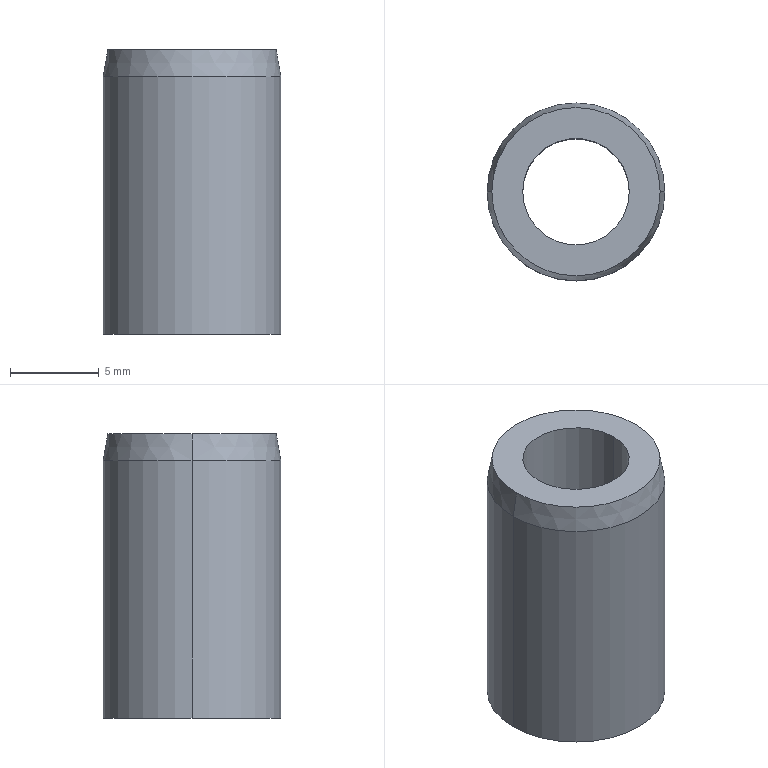Part | STEP file | Probe guide bush JBA6-16 | 1 solid | 10 faces | box 10 x 10 x 16 mm | volume 793.757 mm3 | cylinder 4 | spline 2 | cone 2 | plane 2 | commonest cylinder face diameters 6 x2 10 x2
STEP:
#1=CARTESIAN_POINT('',(0.,0.,0.));
#2=DIRECTION('',(0.,0.,1.));
#3=DIRECTION('',(1.,0.,0.));
#4=AXIS2_PLACEMENT_3D('',#1,#2,#3);
#5=CARTESIAN_POINT('',(4.,0.,0.));
#6=VERTEX_POINT('',#5);
#7=CARTESIAN_POINT('',(-4.,0.,0.));
#8=VERTEX_POINT('',#7);
#9=CARTESIAN_POINT('',(4.,0.,0.));
#10=CARTESIAN_POINT('',(4.,-8.,0.));
#11=CARTESIAN_POINT('',(-4.,-8.,0.));
#12=CARTESIAN_POINT('',(-4.,0.,0.));
#13=(BOUNDED_CURVE()B_SPLINE_CURVE(3,(#9,#10,#11,#12),.UNSPECIFIED.,.F.,.F.)B_SPLINE_CURVE_WITH_KNOTS((4,4),(0.,1.),.PIECEWISE_BEZIER_KNOTS.)CURVE()GEOMETRIC_REPRESENTATION_ITEM()RATIONAL_B_SPLINE_CURVE((1.,0.3333,0.3333,1.))REPRESENTATION_ITEM(''));
#14=CARTESIAN_POINT('',(-4.,0.,0.));
#15=CARTESIAN_POINT('',(-4.,-8.,0.));
#16=CARTESIAN_POINT('',(4.,-8.,0.));
#17=CARTESIAN_POINT('',(4.,0.,0.));
#18=CARTESIAN_POINT('',(-3.414,0.,0.));
#19=CARTESIAN_POINT('',(-3.414,-6.828,0.));
#20=CARTESIAN_POINT('',(3.414,-6.828,0.));
#21=CARTESIAN_POINT('',(3.414,0.,0.));
#22=CARTESIAN_POINT('',(-3.,0.,0.4142));
#23=CARTESIAN_POINT('',(-3.,-6.,0.4142));
#24=CARTESIAN_POINT('',(3.,-6.,0.4142));
#25=CARTESIAN_POINT('',(3.,0.,0.4142));
#26=CARTESIAN_POINT('',(-3.,0.,1.));
#27=CARTESIAN_POINT('',(-3.,-6.,1.));
#28=CARTESIAN_POINT('',(3.,-6.,1.));
#29=CARTESIAN_POINT('',(3.,0.,1.));
#30=(BOUNDED_SURFACE()B_SPLINE_SURFACE(3,3,((#14,#15,#16,#17),(#18,#19,#20,#21),(#22,#23,#24,#25),(#26,#27,#28,#29)),.UNSPECIFIED.,.F.,.F.,.F.)B_SPLINE_SURFACE_WITH_KNOTS((4,4),(4,4),(0.,1.),(0.,1.),.PIECEWISE_BEZIER_KNOTS.)GEOMETRIC_REPRESENTATION_ITEM()RATIONAL_B_SPLINE_SURFACE(((1.,0.3333,0.3333,1.),(0.8047,0.2682,0.2682,0.8047),(0.8047,0.2682,0.2682,0.8047),(1.,0.3333,0.3333,1.)))REPRESENTATION_ITEM('')SURFACE());
#31=CARTESIAN_POINT('',(0.,1.));
#32=DIRECTION('',(0.,-1.));
#33=VECTOR('',#32,1.);
#34=LINE('',#31,#33);
#35=(GEOMETRIC_REPRESENTATION_CONTEXT(2)PARAMETRIC_REPRESENTATION_CONTEXT()REPRESENTATION_CONTEXT('',''));
#36=DEFINITIONAL_REPRESENTATION('',(#34),#35);
#37=PCURVE('',#30,#36);
#38=CARTESIAN_POINT('',(0.,0.,0.));
#39=DIRECTION('',(0.,0.,1.));
#40=DIRECTION('',(1.,0.,0.));
#41=AXIS2_PLACEMENT_3D('',#38,#39,#40);
#42=PLANE('',#41);
#43=CARTESIAN_POINT('',(4.,0.));
#44=CARTESIAN_POINT('',(4.,-8.));
#45=CARTESIAN_POINT('',(-4.,-8.));
#46=CARTESIAN_POINT('',(-4.,0.));
#47=(BOUNDED_CURVE()B_SPLINE_CURVE(3,(#43,#44,#45,#46),.UNSPECIFIED.,.F.,.F.)B_SPLINE_CURVE_WITH_KNOTS((4,4),(0.,1.),.PIECEWISE_BEZIER_KNOTS.)CURVE()GEOMETRIC_REPRESENTATION_ITEM()RATIONAL_B_SPLINE_CURVE((1.,0.3333,0.3333,1.))REPRESENTATION_ITEM(''));
#48=(GEOMETRIC_REPRESENTATION_CONTEXT(2)PARAMETRIC_REPRESENTATION_CONTEXT()REPRESENTATION_CONTEXT('',''));
#49=DEFINITIONAL_REPRESENTATION('',(#47),#48);
#50=PCURVE('',#42,#49);
#51=SURFACE_CURVE('',#13,(#37,#50),.PCURVE_S1.);
#52=EDGE_CURVE('',#6,#8,#51,.T.);
#53=ORIENTED_EDGE('',*,*,#52,.T.);
#54=CARTESIAN_POINT('',(-3.,0.,1.));
#55=VERTEX_POINT('',#54);
#56=CARTESIAN_POINT('',(-4.,0.,1.));
#57=DIRECTION('',(0.,-1.,0.));
#58=DIRECTION('',(-1.,0.,0.));
#59=AXIS2_PLACEMENT_3D('',#56,#57,#58);
#60=CIRCLE('',#59,1.);
#61=CARTESIAN_POINT('',(0.,0.));
#62=CARTESIAN_POINT('',(0.01683,0.));
#63=CARTESIAN_POINT('',(0.04999,0.));
#64=CARTESIAN_POINT('',(0.09843,0.));
#65=CARTESIAN_POINT('',(0.1457,0.));
#66=CARTESIAN_POINT('',(0.192,0.));
#67=CARTESIAN_POINT('',(0.2375,0.));
#68=CARTESIAN_POINT('',(0.2823,0.));
#69=CARTESIAN_POINT('',(0.3265,0.));
#70=CARTESIAN_POINT('',(0.3703,0.));
#71=CARTESIAN_POINT('',(0.4137,0.));
#72=CARTESIAN_POINT('',(0.4569,0.));
#73=CARTESIAN_POINT('',(0.5,0.));
#74=CARTESIAN_POINT('',(0.5431,0.));
#75=CARTESIAN_POINT('',(0.5863,0.));
#76=CARTESIAN_POINT('',(0.6297,0.));
#77=CARTESIAN_POINT('',(0.6735,0.));
#78=CARTESIAN_POINT('',(0.7177,0.));
#79=CARTESIAN_POINT('',(0.7625,0.));
#80=CARTESIAN_POINT('',(0.808,0.));
#81=CARTESIAN_POINT('',(0.8543,0.));
#82=CARTESIAN_POINT('',(0.9016,0.));
#83=CARTESIAN_POINT('',(0.95,0.));
#84=CARTESIAN_POINT('',(0.9832,0.));
#85=CARTESIAN_POINT('',(1.,0.));
#86=B_SPLINE_CURVE_WITH_KNOTS('',3,(#61,#62,#63,#64,#65,#66,#67,#68,#69,#70,#71,#72,#73,#74,#75,#76,#77,#78,#79,#80,#81,#82,#83,#84,#85),.UNSPECIFIED.,.F.,.F.,(4,1,1,1,1,1,1,1,1,1,1,1,1,1,1,1,1,1,1,1,1,1,4),(1.571,1.642,1.714,1.785,1.856,1.928,1.999,2.071,2.142,2.213,2.285,2.356,2.428,2.499,2.57,2.642,2.713,2.785,2.856,2.927,2.999,3.07,3.142),.QUASI_UNIFORM_KNOTS.);
#87=(GEOMETRIC_REPRESENTATION_CONTEXT(2)PARAMETRIC_REPRESENTATION_CONTEXT()REPRESENTATION_CONTEXT('',''));
#88=DEFINITIONAL_REPRESENTATION('',(#86),#87);
#89=PCURVE('',#30,#88);
#90=CARTESIAN_POINT('',(4.,0.,0.));
#91=CARTESIAN_POINT('',(4.,8.,0.));
#92=CARTESIAN_POINT('',(-4.,8.,0.));
#93=CARTESIAN_POINT('',(-4.,0.,0.));
#94=CARTESIAN_POINT('',(3.414,0.,0.));
#95=CARTESIAN_POINT('',(3.414,6.828,0.));
#96=CARTESIAN_POINT('',(-3.414,6.828,0.));
#97=CARTESIAN_POINT('',(-3.414,0.,0.));
#98=CARTESIAN_POINT('',(3.,0.,0.4142));
#99=CARTESIAN_POINT('',(3.,6.,0.4142));
#100=CARTESIAN_POINT('',(-3.,6.,0.4142));
#101=CARTESIAN_POINT('',(-3.,0.,0.4142));
#102=CARTESIAN_POINT('',(3.,0.,1.));
#103=CARTESIAN_POINT('',(3.,6.,1.));
#104=CARTESIAN_POINT('',(-3.,6.,1.));
#105=CARTESIAN_POINT('',(-3.,0.,1.));
#106=(BOUNDED_SURFACE()B_SPLINE_SURFACE(3,3,((#90,#91,#92,#93),(#94,#95,#96,#97),(#98,#99,#100,#101),(#102,#103,#104,#105)),.UNSPECIFIED.,.F.,.F.,.F.)B_SPLINE_SURFACE_WITH_KNOTS((4,4),(4,4),(0.,1.),(0.,1.),.PIECEWISE_BEZIER_KNOTS.)GEOMETRIC_REPRESENTATION_ITEM()RATIONAL_B_SPLINE_SURFACE(((1.,0.3333,0.3333,1.),(0.8047,0.2682,0.2682,0.8047),(0.8047,0.2682,0.2682,0.8047),(1.,0.3333,0.3333,1.)))REPRESENTATION_ITEM('')SURFACE());
#107=CARTESIAN_POINT('',(0.,1.));
#108=CARTESIAN_POINT('',(0.01683,1.));
#109=CARTESIAN_POINT('',(0.04999,1.));
#110=CARTESIAN_POINT('',(0.09843,1.));
#111=CARTESIAN_POINT('',(0.1457,1.));
#112=CARTESIAN_POINT('',(0.192,1.));
#113=CARTESIAN_POINT('',(0.2375,1.));
#114=CARTESIAN_POINT('',(0.2823,1.));
#115=CARTESIAN_POINT('',(0.3265,1.));
#116=CARTESIAN_POINT('',(0.3703,1.));
#117=CARTESIAN_POINT('',(0.4137,1.));
#118=CARTESIAN_POINT('',(0.4569,1.));
#119=CARTESIAN_POINT('',(0.5,1.));
#120=CARTESIAN_POINT('',(0.5431,1.));
#121=CARTESIAN_POINT('',(0.5863,1.));
#122=CARTESIAN_POINT('',(0.6297,1.));
#123=CARTESIAN_POINT('',(0.6735,1.));
#124=CARTESIAN_POINT('',(0.7177,1.));
#125=CARTESIAN_POINT('',(0.7625,1.));
#126=CARTESIAN_POINT('',(0.808,1.));
#127=CARTESIAN_POINT('',(0.8543,1.));
#128=CARTESIAN_POINT('',(0.9016,1.));
#129=CARTESIAN_POINT('',(0.95,1.));
#130=CARTESIAN_POINT('',(0.9832,1.));
#131=CARTESIAN_POINT('',(1.,1.));
#132=B_SPLINE_CURVE_WITH_KNOTS('',3,(#107,#108,#109,#110,#111,#112,#113,#114,#115,#116,#117,#118,#119,#120,#121,#122,#123,#124,#125,#126,#127,#128,#129,#130,#131),.UNSPECIFIED.,.F.,.F.,(4,1,1,1,1,1,1,1,1,1,1,1,1,1,1,1,1,1,1,1,1,1,4),(1.571,1.642,1.714,1.785,1.856,1.928,1.999,2.071,2.142,2.213,2.285,2.356,2.428,2.499,2.57,2.642,2.713,2.785,2.856,2.927,2.999,3.07,3.142),.QUASI_UNIFORM_KNOTS.);
#133=(GEOMETRIC_REPRESENTATION_CONTEXT(2)PARAMETRIC_REPRESENTATION_CONTEXT()REPRESENTATION_CONTEXT('',''));
#134=DEFINITIONAL_REPRESENTATION('',(#132),#133);
#135=PCURVE('',#106,#134);
#136=SURFACE_CURVE('',#60,(#89,#135),.PCURVE_S1.);
#137=EDGE_CURVE('',#8,#55,#136,.T.);
#138=ORIENTED_EDGE('',*,*,#137,.T.);
#139=CARTESIAN_POINT('',(3.,0.,1.));
#140=VERTEX_POINT('',#139);
#141=CARTESIAN_POINT('',(0.,0.,1.));
#142=DIRECTION('',(0.,0.,1.));
#143=DIRECTION('',(1.,0.,0.));
#144=AXIS2_PLACEMENT_3D('',#141,#142,#143);
#145=CIRCLE('',#144,3.);
#146=CARTESIAN_POINT('',(1.,0.));
#147=CARTESIAN_POINT('',(1.,0.02375));
#148=CARTESIAN_POINT('',(1.,0.06805));
#149=CARTESIAN_POINT('',(1.,0.1267));
#150=CARTESIAN_POINT('',(1.,0.1794));
#151=CARTESIAN_POINT('',(1.,0.2276));
#152=CARTESIAN_POINT('',(1.,0.2721));
#153=CARTESIAN_POINT('',(1.,0.3139));
#154=CARTESIAN_POINT('',(1.,0.3535));
#155=CARTESIAN_POINT('',(1.,0.3914));
#156=CARTESIAN_POINT('',(1.,0.4282));
#157=CARTESIAN_POINT('',(1.,0.4643));
#158=CARTESIAN_POINT('',(1.,0.5));
#159=CARTESIAN_POINT('',(1.,0.5357));
#160=CARTESIAN_POINT('',(1.,0.5718));
#161=CARTESIAN_POINT('',(1.,0.6086));
#162=CARTESIAN_POINT('',(1.,0.6465));
#163=CARTESIAN_POINT('',(1.,0.6861));
#164=CARTESIAN_POINT('',(1.,0.7279));
#165=CARTESIAN_POINT('',(1.,0.7724));
#166=CARTESIAN_POINT('',(1.,0.8206));
#167=CARTESIAN_POINT('',(1.,0.8733));
#168=CARTESIAN_POINT('',(1.,0.9319));
#169=CARTESIAN_POINT('',(1.,0.9763));
#170=CARTESIAN_POINT('',(1.,1.));
#171=B_SPLINE_CURVE_WITH_KNOTS('',3,(#146,#147,#148,#149,#150,#151,#152,#153,#154,#155,#156,#157,#158,#159,#160,#161,#162,#163,#164,#165,#166,#167,#168,#169,#170),.UNSPECIFIED.,.F.,.F.,(4,1,1,1,1,1,1,1,1,1,1,1,1,1,1,1,1,1,1,1,1,1,4),(3.142,3.284,3.427,3.57,3.713,3.856,3.998,4.141,4.284,4.427,4.57,4.712,4.855,4.998,5.141,5.284,5.426,5.569,5.712,5.855,5.998,6.14,6.283),.QUASI_UNIFORM_KNOTS.);
#172=(GEOMETRIC_REPRESENTATION_CONTEXT(2)PARAMETRIC_REPRESENTATION_CONTEXT()REPRESENTATION_CONTEXT('',''));
#173=DEFINITIONAL_REPRESENTATION('',(#171),#172);
#174=PCURVE('',#30,#173);
#175=CARTESIAN_POINT('',(0.,0.,16.));
#176=DIRECTION('',(0.,0.,-1.));
#177=DIRECTION('',(-1.,0.,0.));
#178=AXIS2_PLACEMENT_3D('',#175,#176,#177);
#179=CYLINDRICAL_SURFACE('',#178,3.);
#180=CARTESIAN_POINT('',(9.425,15.));
#181=DIRECTION('',(-1.,0.));
#182=VECTOR('',#181,1.);
#183=LINE('',#180,#182);
#184=(GEOMETRIC_REPRESENTATION_CONTEXT(2)PARAMETRIC_REPRESENTATION_CONTEXT()REPRESENTATION_CONTEXT('',''));
#185=DEFINITIONAL_REPRESENTATION('',(#183),#184);
#186=PCURVE('',#179,#185);
#187=SURFACE_CURVE('',#145,(#174,#186),.PCURVE_S1.);
#188=EDGE_CURVE('',#55,#140,#187,.T.);
#189=ORIENTED_EDGE('',*,*,#188,.T.);
#190=CARTESIAN_POINT('',(4.,0.,1.));
#191=DIRECTION('',(0.,1.,0.));
#192=DIRECTION('',(1.,0.,0.));
#193=AXIS2_PLACEMENT_3D('',#190,#191,#192);
#194=CIRCLE('',#193,1.);
#195=CARTESIAN_POINT('',(0.,1.));
#196=CARTESIAN_POINT('',(0.01683,1.));
#197=CARTESIAN_POINT('',(0.04999,1.));
#198=CARTESIAN_POINT('',(0.09843,1.));
#199=CARTESIAN_POINT('',(0.1457,1.));
#200=CARTESIAN_POINT('',(0.192,1.));
#201=CARTESIAN_POINT('',(0.2375,1.));
#202=CARTESIAN_POINT('',(0.2823,1.));
#203=CARTESIAN_POINT('',(0.3265,1.));
#204=CARTESIAN_POINT('',(0.3703,1.));
#205=CARTESIAN_POINT('',(0.4137,1.));
#206=CARTESIAN_POINT('',(0.4569,1.));
#207=CARTESIAN_POINT('',(0.5,1.));
#208=CARTESIAN_POINT('',(0.5431,1.));
#209=CARTESIAN_POINT('',(0.5863,1.));
#210=CARTESIAN_POINT('',(0.6297,1.));
#211=CARTESIAN_POINT('',(0.6735,1.));
#212=CARTESIAN_POINT('',(0.7177,1.));
#213=CARTESIAN_POINT('',(0.7625,1.));
#214=CARTESIAN_POINT('',(0.808,1.));
#215=CARTESIAN_POINT('',(0.8543,1.));
#216=CARTESIAN_POINT('',(0.9016,1.));
#217=CARTESIAN_POINT('',(0.95,1.));
#218=CARTESIAN_POINT('',(0.9832,1.));
#219=CARTESIAN_POINT('',(1.,1.));
#220=B_SPLINE_CURVE_WITH_KNOTS('',3,(#195,#196,#197,#198,#199,#200,#201,#202,#203,#204,#205,#206,#207,#208,#209,#210,#211,#212,#213,#214,#215,#216,#217,#218,#219),.UNSPECIFIED.,.F.,.F.,(4,1,1,1,1,1,1,1,1,1,1,1,1,1,1,1,1,1,1,1,1,1,4),(1.571,1.642,1.714,1.785,1.856,1.928,1.999,2.071,2.142,2.213,2.285,2.356,2.428,2.499,2.57,2.642,2.713,2.785,2.856,2.927,2.999,3.07,3.142),.QUASI_UNIFORM_KNOTS.);
#221=(GEOMETRIC_REPRESENTATION_CONTEXT(2)PARAMETRIC_REPRESENTATION_CONTEXT()REPRESENTATION_CONTEXT('',''));
#222=DEFINITIONAL_REPRESENTATION('',(#220),#221);
#223=PCURVE('',#30,#222);
#224=CARTESIAN_POINT('',(0.,0.));
#225=CARTESIAN_POINT('',(0.01683,0.));
#226=CARTESIAN_POINT('',(0.04999,0.));
#227=CARTESIAN_POINT('',(0.09843,0.));
#228=CARTESIAN_POINT('',(0.1457,0.));
#229=CARTESIAN_POINT('',(0.192,0.));
#230=CARTESIAN_POINT('',(0.2375,0.));
#231=CARTESIAN_POINT('',(0.2823,0.));
#232=CARTESIAN_POINT('',(0.3265,0.));
#233=CARTESIAN_POINT('',(0.3703,0.));
#234=CARTESIAN_POINT('',(0.4137,0.));
#235=CARTESIAN_POINT('',(0.4569,0.));
#236=CARTESIAN_POINT('',(0.5,0.));
#237=CARTESIAN_POINT('',(0.5431,0.));
#238=CARTESIAN_POINT('',(0.5863,0.));
#239=CARTESIAN_POINT('',(0.6297,0.));
#240=CARTESIAN_POINT('',(0.6735,0.));
#241=CARTESIAN_POINT('',(0.7177,0.));
#242=CARTESIAN_POINT('',(0.7625,0.));
#243=CARTESIAN_POINT('',(0.808,0.));
#244=CARTESIAN_POINT('',(0.8543,0.));
#245=CARTESIAN_POINT('',(0.9016,0.));
#246=CARTESIAN_POINT('',(0.95,0.));
#247=CARTESIAN_POINT('',(0.9832,0.));
#248=CARTESIAN_POINT('',(1.,0.));
#249=B_SPLINE_CURVE_WITH_KNOTS('',3,(#224,#225,#226,#227,#228,#229,#230,#231,#232,#233,#234,#235,#236,#237,#238,#239,#240,#241,#242,#243,#244,#245,#246,#247,#248),.UNSPECIFIED.,.F.,.F.,(4,1,1,1,1,1,1,1,1,1,1,1,1,1,1,1,1,1,1,1,1,1,4),(1.571,1.642,1.714,1.785,1.856,1.928,1.999,2.071,2.142,2.213,2.285,2.356,2.428,2.499,2.57,2.642,2.713,2.785,2.856,2.927,2.999,3.07,3.142),.QUASI_UNIFORM_KNOTS.);
#250=(GEOMETRIC_REPRESENTATION_CONTEXT(2)PARAMETRIC_REPRESENTATION_CONTEXT()REPRESENTATION_CONTEXT('',''));
#251=DEFINITIONAL_REPRESENTATION('',(#249),#250);
#252=PCURVE('',#106,#251);
#253=SURFACE_CURVE('',#194,(#223,#252),.PCURVE_S1.);
#254=EDGE_CURVE('',#6,#140,#253,.T.);
#255=ORIENTED_EDGE('',*,*,#254,.F.);
#256=EDGE_LOOP('',(#53,#138,#189,#255));
#257=FACE_BOUND('',#256,.T.);
#258=ADVANCED_FACE('',(#257),#30,.T.);
#259=CARTESIAN_POINT('',(-5.,0.,14.5));
#260=VERTEX_POINT('',#259);
#261=CARTESIAN_POINT('',(5.,0.,14.5));
#262=VERTEX_POINT('',#261);
#263=CARTESIAN_POINT('',(0.,0.,14.5));
#264=DIRECTION('',(0.,0.,-1.));
#265=DIRECTION('',(-1.,0.,0.));
#266=AXIS2_PLACEMENT_3D('',#263,#264,#265);
#267=CIRCLE('',#266,5.);
#268=CARTESIAN_POINT('',(0.,0.,16.));
#269=DIRECTION('',(0.,0.,-1.));
#270=DIRECTION('',(-1.,0.,0.));
#271=AXIS2_PLACEMENT_3D('',#268,#269,#270);
#272=CYLINDRICAL_SURFACE('',#271,5.);
#273=CARTESIAN_POINT('',(0.,1.5));
#274=DIRECTION('',(1.,0.));
#275=VECTOR('',#274,1.);
#276=LINE('',#273,#275);
#277=(GEOMETRIC_REPRESENTATION_CONTEXT(2)PARAMETRIC_REPRESENTATION_CONTEXT()REPRESENTATION_CONTEXT('',''));
#278=DEFINITIONAL_REPRESENTATION('',(#276),#277);
#279=PCURVE('',#272,#278);
#280=CARTESIAN_POINT('',(0.,0.,14.5));
#281=DIRECTION('',(0.,0.,-1.));
#282=DIRECTION('',(-1.,0.,0.));
#283=AXIS2_PLACEMENT_3D('',#280,#281,#282);
#284=CONICAL_SURFACE('',#283,5.,0.1745);
#285=CARTESIAN_POINT('',(0.,0.));
#286=DIRECTION('',(1.,0.));
#287=VECTOR('',#286,1.);
#288=LINE('',#285,#287);
#289=(GEOMETRIC_REPRESENTATION_CONTEXT(2)PARAMETRIC_REPRESENTATION_CONTEXT()REPRESENTATION_CONTEXT('',''));
#290=DEFINITIONAL_REPRESENTATION('',(#288),#289);
#291=PCURVE('',#284,#290);
#292=SURFACE_CURVE('',#267,(#279,#291),.PCURVE_S1.);
#293=EDGE_CURVE('',#260,#262,#292,.T.);
#294=ORIENTED_EDGE('',*,*,#293,.T.);
#295=CARTESIAN_POINT('',(5.,0.,0.));
#296=VERTEX_POINT('',#295);
#297=CARTESIAN_POINT('',(5.,0.,16.));
#298=DIRECTION('',(0.,0.,-1.));
#299=VECTOR('',#298,1.);
#300=LINE('',#297,#299);
#301=CARTESIAN_POINT('',(3.142,0.));
#302=DIRECTION('',(0.,1.));
#303=VECTOR('',#302,1.);
#304=LINE('',#301,#303);
#305=(GEOMETRIC_REPRESENTATION_CONTEXT(2)PARAMETRIC_REPRESENTATION_CONTEXT()REPRESENTATION_CONTEXT('',''));
#306=DEFINITIONAL_REPRESENTATION('',(#304),#305);
#307=PCURVE('',#272,#306);
#308=CARTESIAN_POINT('',(0.,0.,16.));
#309=DIRECTION('',(0.,0.,-1.));
#310=DIRECTION('',(-1.,0.,0.));
#311=AXIS2_PLACEMENT_3D('',#308,#309,#310);
#312=CYLINDRICAL_SURFACE('',#311,5.);
#313=CARTESIAN_POINT('',(3.142,0.));
#314=DIRECTION('',(0.,1.));
#315=VECTOR('',#314,1.);
#316=LINE('',#313,#315);
#317=(GEOMETRIC_REPRESENTATION_CONTEXT(2)PARAMETRIC_REPRESENTATION_CONTEXT()REPRESENTATION_CONTEXT('',''));
#318=DEFINITIONAL_REPRESENTATION('',(#316),#317);
#319=PCURVE('',#312,#318);
#320=SURFACE_CURVE('',#300,(#307,#319),.PCURVE_S1.);
#321=EDGE_CURVE('',#262,#296,#320,.T.);
#322=ORIENTED_EDGE('',*,*,#321,.T.);
#323=CARTESIAN_POINT('',(-5.,0.,0.));
#324=VERTEX_POINT('',#323);
#325=CARTESIAN_POINT('',(0.,0.,0.));
#326=DIRECTION('',(0.,0.,1.));
#327=DIRECTION('',(-1.,0.,0.));
#328=AXIS2_PLACEMENT_3D('',#325,#326,#327);
#329=CIRCLE('',#328,5.);
#330=CARTESIAN_POINT('',(6.283,16.));
#331=DIRECTION('',(-1.,0.));
#332=VECTOR('',#331,1.);
#333=LINE('',#330,#332);
#334=(GEOMETRIC_REPRESENTATION_CONTEXT(2)PARAMETRIC_REPRESENTATION_CONTEXT()REPRESENTATION_CONTEXT('',''));
#335=DEFINITIONAL_REPRESENTATION('',(#333),#334);
#336=PCURVE('',#272,#335);
#337=CARTESIAN_POINT('',(0.,0.));
#338=DIRECTION('',(-1.,0.));
#339=AXIS2_PLACEMENT_2D('',#337,#338);
#340=CIRCLE('',#339,5.);
#341=(GEOMETRIC_REPRESENTATION_CONTEXT(2)PARAMETRIC_REPRESENTATION_CONTEXT()REPRESENTATION_CONTEXT('',''));
#342=DEFINITIONAL_REPRESENTATION('',(#340),#341);
#343=PCURVE('',#42,#342);
#344=SURFACE_CURVE('',#329,(#336,#343),.PCURVE_S1.);
#345=EDGE_CURVE('',#296,#324,#344,.T.);
#346=ORIENTED_EDGE('',*,*,#345,.T.);
#347=CARTESIAN_POINT('',(-5.,0.,16.));
#348=DIRECTION('',(0.,0.,-1.));
#349=VECTOR('',#348,1.);
#350=LINE('',#347,#349);
#351=CARTESIAN_POINT('',(0.,0.));
#352=DIRECTION('',(0.,1.));
#353=VECTOR('',#352,1.);
#354=LINE('',#351,#353);
#355=(GEOMETRIC_REPRESENTATION_CONTEXT(2)PARAMETRIC_REPRESENTATION_CONTEXT()REPRESENTATION_CONTEXT('',''));
#356=DEFINITIONAL_REPRESENTATION('',(#354),#355);
#357=PCURVE('',#272,#356);
#358=CARTESIAN_POINT('',(6.283,0.));
#359=DIRECTION('',(0.,1.));
#360=VECTOR('',#359,1.);
#361=LINE('',#358,#360);
#362=(GEOMETRIC_REPRESENTATION_CONTEXT(2)PARAMETRIC_REPRESENTATION_CONTEXT()REPRESENTATION_CONTEXT('',''));
#363=DEFINITIONAL_REPRESENTATION('',(#361),#362);
#364=PCURVE('',#312,#363);
#365=SURFACE_CURVE('',#350,(#357,#364),.PCURVE_S1.);
#366=EDGE_CURVE('',#260,#324,#365,.T.);
#367=ORIENTED_EDGE('',*,*,#366,.F.);
#368=EDGE_LOOP('',(#294,#322,#346,#367));
#369=FACE_BOUND('',#368,.T.);
#370=ADVANCED_FACE('',(#369),#272,.T.);
#371=CARTESIAN_POINT('',(-4.736,0.,16.));
#372=VERTEX_POINT('',#371);
#373=CARTESIAN_POINT('',(4.736,0.,16.));
#374=VERTEX_POINT('',#373);
#375=CARTESIAN_POINT('',(0.,0.,16.));
#376=DIRECTION('',(0.,0.,-1.));
#377=DIRECTION('',(-1.,0.,0.));
#378=AXIS2_PLACEMENT_3D('',#375,#376,#377);
#379=CIRCLE('',#378,4.736);
#380=CARTESIAN_POINT('',(0.,-1.5));
#381=DIRECTION('',(1.,0.));
#382=VECTOR('',#381,1.);
#383=LINE('',#380,#382);
#384=(GEOMETRIC_REPRESENTATION_CONTEXT(2)PARAMETRIC_REPRESENTATION_CONTEXT()REPRESENTATION_CONTEXT('',''));
#385=DEFINITIONAL_REPRESENTATION('',(#383),#384);
#386=PCURVE('',#284,#385);
#387=CARTESIAN_POINT('',(0.,0.,16.));
#388=DIRECTION('',(0.,0.,1.));
#389=DIRECTION('',(1.,0.,0.));
#390=AXIS2_PLACEMENT_3D('',#387,#388,#389);
#391=PLANE('',#390);
#392=CARTESIAN_POINT('',(-4.736,0.));
#393=CARTESIAN_POINT('',(-4.736,8.202));
#394=CARTESIAN_POINT('',(2.368,4.101));
#395=CARTESIAN_POINT('',(9.471,0.));
#396=CARTESIAN_POINT('',(2.368,-4.101));
#397=CARTESIAN_POINT('',(-4.736,-8.202));
#398=CARTESIAN_POINT('',(-4.736,0.));
#399=(BOUNDED_CURVE()B_SPLINE_CURVE(2,(#392,#393,#394,#395,#396,#397,#398),.UNSPECIFIED.,.T.,.F.)B_SPLINE_CURVE_WITH_KNOTS((1,2,2,2,2,1),(-2.094,0.,2.094,4.189,6.283,8.378),.UNSPECIFIED.)CURVE()GEOMETRIC_REPRESENTATION_ITEM()RATIONAL_B_SPLINE_CURVE((1.,0.5,1.,0.5,1.,0.5,1.))REPRESENTATION_ITEM(''));
#400=(GEOMETRIC_REPRESENTATION_CONTEXT(2)PARAMETRIC_REPRESENTATION_CONTEXT()REPRESENTATION_CONTEXT('',''));
#401=DEFINITIONAL_REPRESENTATION('',(#399),#400);
#402=PCURVE('',#391,#401);
#403=SURFACE_CURVE('',#379,(#386,#402),.PCURVE_S1.);
#404=EDGE_CURVE('',#372,#374,#403,.T.);
#405=ORIENTED_EDGE('',*,*,#404,.T.);
#406=CARTESIAN_POINT('',(5.,0.,14.5));
#407=DIRECTION('',(0.1736,0.,-0.9848));
#408=VECTOR('',#407,1.);
#409=LINE('',#406,#408);
#410=CARTESIAN_POINT('',(3.142,0.));
#411=DIRECTION('',(0.,1.));
#412=VECTOR('',#411,1.);
#413=LINE('',#410,#412);
#414=(GEOMETRIC_REPRESENTATION_CONTEXT(2)PARAMETRIC_REPRESENTATION_CONTEXT()REPRESENTATION_CONTEXT('',''));
#415=DEFINITIONAL_REPRESENTATION('',(#413),#414);
#416=PCURVE('',#284,#415);
#417=CARTESIAN_POINT('',(0.,0.,14.5));
#418=DIRECTION('',(0.,0.,-1.));
#419=DIRECTION('',(-1.,0.,0.));
#420=AXIS2_PLACEMENT_3D('',#417,#418,#419);
#421=CONICAL_SURFACE('',#420,5.,0.1745);
#422=CARTESIAN_POINT('',(3.142,0.));
#423=DIRECTION('',(0.,1.));
#424=VECTOR('',#423,1.);
#425=LINE('',#422,#424);
#426=(GEOMETRIC_REPRESENTATION_CONTEXT(2)PARAMETRIC_REPRESENTATION_CONTEXT()REPRESENTATION_CONTEXT('',''));
#427=DEFINITIONAL_REPRESENTATION('',(#425),#426);
#428=PCURVE('',#421,#427);
#429=SURFACE_CURVE('',#409,(#416,#428),.PCURVE_S1.);
#430=EDGE_CURVE('',#374,#262,#429,.T.);
#431=ORIENTED_EDGE('',*,*,#430,.T.);
#432=ORIENTED_EDGE('',*,*,#293,.F.);
#433=CARTESIAN_POINT('',(-5.,0.,14.5));
#434=DIRECTION('',(-0.1736,0.,-0.9848));
#435=VECTOR('',#434,1.);
#436=LINE('',#433,#435);
#437=CARTESIAN_POINT('',(0.,0.));
#438=DIRECTION('',(0.,1.));
#439=VECTOR('',#438,1.);
#440=LINE('',#437,#439);
#441=(GEOMETRIC_REPRESENTATION_CONTEXT(2)PARAMETRIC_REPRESENTATION_CONTEXT()REPRESENTATION_CONTEXT('',''));
#442=DEFINITIONAL_REPRESENTATION('',(#440),#441);
#443=PCURVE('',#284,#442);
#444=CARTESIAN_POINT('',(6.283,0.));
#445=DIRECTION('',(0.,1.));
#446=VECTOR('',#445,1.);
#447=LINE('',#444,#446);
#448=(GEOMETRIC_REPRESENTATION_CONTEXT(2)PARAMETRIC_REPRESENTATION_CONTEXT()REPRESENTATION_CONTEXT('',''));
#449=DEFINITIONAL_REPRESENTATION('',(#447),#448);
#450=PCURVE('',#421,#449);
#451=SURFACE_CURVE('',#436,(#443,#450),.PCURVE_S1.);
#452=EDGE_CURVE('',#372,#260,#451,.T.);
#453=ORIENTED_EDGE('',*,*,#452,.F.);
#454=EDGE_LOOP('',(#405,#431,#432,#453));
#455=FACE_BOUND('',#454,.T.);
#456=ADVANCED_FACE('',(#455),#284,.T.);
#457=CARTESIAN_POINT('',(-3.,0.,16.));
#458=VERTEX_POINT('',#457);
#459=CARTESIAN_POINT('',(-3.,0.,16.));
#460=DIRECTION('',(0.,0.,-1.));
#461=VECTOR('',#460,1.);
#462=LINE('',#459,#461);
#463=CARTESIAN_POINT('',(6.283,0.));
#464=DIRECTION('',(0.,1.));
#465=VECTOR('',#464,1.);
#466=LINE('',#463,#465);
#467=(GEOMETRIC_REPRESENTATION_CONTEXT(2)PARAMETRIC_REPRESENTATION_CONTEXT()REPRESENTATION_CONTEXT('',''));
#468=DEFINITIONAL_REPRESENTATION('',(#466),#467);
#469=PCURVE('',#179,#468);
#470=CARTESIAN_POINT('',(0.,0.,16.));
#471=DIRECTION('',(0.,0.,-1.));
#472=DIRECTION('',(-1.,0.,0.));
#473=AXIS2_PLACEMENT_3D('',#470,#471,#472);
#474=CYLINDRICAL_SURFACE('',#473,3.);
#475=CARTESIAN_POINT('',(0.,0.));
#476=DIRECTION('',(0.,1.));
#477=VECTOR('',#476,1.);
#478=LINE('',#475,#477);
#479=(GEOMETRIC_REPRESENTATION_CONTEXT(2)PARAMETRIC_REPRESENTATION_CONTEXT()REPRESENTATION_CONTEXT('',''));
#480=DEFINITIONAL_REPRESENTATION('',(#478),#479);
#481=PCURVE('',#474,#480);
#482=SURFACE_CURVE('',#462,(#469,#481),.PCURVE_S1.);
#483=EDGE_CURVE('',#458,#55,#482,.T.);
#484=ORIENTED_EDGE('',*,*,#483,.T.);
#485=ORIENTED_EDGE('',*,*,#188,.T.);
#486=CARTESIAN_POINT('',(3.,0.,16.));
#487=VERTEX_POINT('',#486);
#488=CARTESIAN_POINT('',(3.,0.,16.));
#489=DIRECTION('',(0.,0.,-1.));
#490=VECTOR('',#489,1.);
#491=LINE('',#488,#490);
#492=CARTESIAN_POINT('',(3.142,0.));
#493=DIRECTION('',(0.,1.));
#494=VECTOR('',#493,1.);
#495=LINE('',#492,#494);
#496=(GEOMETRIC_REPRESENTATION_CONTEXT(2)PARAMETRIC_REPRESENTATION_CONTEXT()REPRESENTATION_CONTEXT('',''));
#497=DEFINITIONAL_REPRESENTATION('',(#495),#496);
#498=PCURVE('',#179,#497);
#499=CARTESIAN_POINT('',(3.142,0.));
#500=DIRECTION('',(0.,1.));
#501=VECTOR('',#500,1.);
#502=LINE('',#499,#501);
#503=(GEOMETRIC_REPRESENTATION_CONTEXT(2)PARAMETRIC_REPRESENTATION_CONTEXT()REPRESENTATION_CONTEXT('',''));
#504=DEFINITIONAL_REPRESENTATION('',(#502),#503);
#505=PCURVE('',#474,#504);
#506=SURFACE_CURVE('',#491,(#498,#505),.PCURVE_S1.);
#507=EDGE_CURVE('',#487,#140,#506,.T.);
#508=ORIENTED_EDGE('',*,*,#507,.F.);
#509=CARTESIAN_POINT('',(0.,0.,16.));
#510=DIRECTION('',(0.,0.,-1.));
#511=DIRECTION('',(-1.,0.,0.));
#512=AXIS2_PLACEMENT_3D('',#509,#510,#511);
#513=CIRCLE('',#512,3.);
#514=CARTESIAN_POINT('',(0.,0.));
#515=DIRECTION('',(1.,0.));
#516=VECTOR('',#515,1.);
#517=LINE('',#514,#516);
#518=(GEOMETRIC_REPRESENTATION_CONTEXT(2)PARAMETRIC_REPRESENTATION_CONTEXT()REPRESENTATION_CONTEXT('',''));
#519=DEFINITIONAL_REPRESENTATION('',(#517),#518);
#520=PCURVE('',#179,#519);
#521=CARTESIAN_POINT('',(-3.,0.));
#522=CARTESIAN_POINT('',(-3.,5.196));
#523=CARTESIAN_POINT('',(1.5,2.598));
#524=CARTESIAN_POINT('',(6.,0.));
#525=CARTESIAN_POINT('',(1.5,-2.598));
#526=CARTESIAN_POINT('',(-3.,-5.196));
#527=CARTESIAN_POINT('',(-3.,0.));
#528=(BOUNDED_CURVE()B_SPLINE_CURVE(2,(#521,#522,#523,#524,#525,#526,#527),.UNSPECIFIED.,.T.,.F.)B_SPLINE_CURVE_WITH_KNOTS((1,2,2,2,2,1),(-2.094,0.,2.094,4.189,6.283,8.378),.UNSPECIFIED.)CURVE()GEOMETRIC_REPRESENTATION_ITEM()RATIONAL_B_SPLINE_CURVE((1.,0.5,1.,0.5,1.,0.5,1.))REPRESENTATION_ITEM(''));
#529=(GEOMETRIC_REPRESENTATION_CONTEXT(2)PARAMETRIC_REPRESENTATION_CONTEXT()REPRESENTATION_CONTEXT('',''));
#530=DEFINITIONAL_REPRESENTATION('',(#528),#529);
#531=PCURVE('',#391,#530);
#532=SURFACE_CURVE('',#513,(#520,#531),.PCURVE_S1.);
#533=EDGE_CURVE('',#487,#458,#532,.T.);
#534=ORIENTED_EDGE('',*,*,#533,.T.);
#535=EDGE_LOOP('',(#484,#485,#508,#534));
#536=FACE_BOUND('',#535,.F.);
#537=ADVANCED_FACE('',(#536),#179,.F.);
#538=ORIENTED_EDGE('',*,*,#321,.F.);
#539=CARTESIAN_POINT('',(0.,0.,14.5));
#540=DIRECTION('',(0.,0.,-1.));
#541=DIRECTION('',(-1.,0.,0.));
#542=AXIS2_PLACEMENT_3D('',#539,#540,#541);
#543=CIRCLE('',#542,5.);
#544=CARTESIAN_POINT('',(0.,1.5));
#545=DIRECTION('',(1.,0.));
#546=VECTOR('',#545,1.);
#547=LINE('',#544,#546);
#548=(GEOMETRIC_REPRESENTATION_CONTEXT(2)PARAMETRIC_REPRESENTATION_CONTEXT()REPRESENTATION_CONTEXT('',''));
#549=DEFINITIONAL_REPRESENTATION('',(#547),#548);
#550=PCURVE('',#312,#549);
#551=CARTESIAN_POINT('',(0.,0.));
#552=DIRECTION('',(1.,0.));
#553=VECTOR('',#552,1.);
#554=LINE('',#551,#553);
#555=(GEOMETRIC_REPRESENTATION_CONTEXT(2)PARAMETRIC_REPRESENTATION_CONTEXT()REPRESENTATION_CONTEXT('',''));
#556=DEFINITIONAL_REPRESENTATION('',(#554),#555);
#557=PCURVE('',#421,#556);
#558=SURFACE_CURVE('',#543,(#550,#557),.PCURVE_S1.);
#559=EDGE_CURVE('',#262,#260,#558,.T.);
#560=ORIENTED_EDGE('',*,*,#559,.T.);
#561=ORIENTED_EDGE('',*,*,#366,.T.);
#562=CARTESIAN_POINT('',(0.,0.,0.));
#563=DIRECTION('',(0.,0.,1.));
#564=DIRECTION('',(-1.,0.,0.));
#565=AXIS2_PLACEMENT_3D('',#562,#563,#564);
#566=CIRCLE('',#565,5.);
#567=CARTESIAN_POINT('',(6.283,16.));
#568=DIRECTION('',(-1.,0.));
#569=VECTOR('',#568,1.);
#570=LINE('',#567,#569);
#571=(GEOMETRIC_REPRESENTATION_CONTEXT(2)PARAMETRIC_REPRESENTATION_CONTEXT()REPRESENTATION_CONTEXT('',''));
#572=DEFINITIONAL_REPRESENTATION('',(#570),#571);
#573=PCURVE('',#312,#572);
#574=CARTESIAN_POINT('',(0.,0.));
#575=DIRECTION('',(-1.,0.));
#576=AXIS2_PLACEMENT_2D('',#574,#575);
#577=CIRCLE('',#576,5.);
#578=(GEOMETRIC_REPRESENTATION_CONTEXT(2)PARAMETRIC_REPRESENTATION_CONTEXT()REPRESENTATION_CONTEXT('',''));
#579=DEFINITIONAL_REPRESENTATION('',(#577),#578);
#580=PCURVE('',#42,#579);
#581=SURFACE_CURVE('',#566,(#573,#580),.PCURVE_S1.);
#582=EDGE_CURVE('',#324,#296,#581,.T.);
#583=ORIENTED_EDGE('',*,*,#582,.T.);
#584=EDGE_LOOP('',(#538,#560,#561,#583));
#585=FACE_BOUND('',#584,.T.);
#586=ADVANCED_FACE('',(#585),#312,.T.);
#587=ORIENTED_EDGE('',*,*,#582,.F.);
#588=ORIENTED_EDGE('',*,*,#345,.F.);
#589=EDGE_LOOP('',(#587,#588));
#590=FACE_BOUND('',#589,.T.);
#591=ORIENTED_EDGE('',*,*,#52,.F.);
#592=CARTESIAN_POINT('',(-4.,0.,0.));
#593=CARTESIAN_POINT('',(-4.,8.,0.));
#594=CARTESIAN_POINT('',(4.,8.,0.));
#595=CARTESIAN_POINT('',(4.,0.,0.));
#596=(BOUNDED_CURVE()B_SPLINE_CURVE(3,(#592,#593,#594,#595),.UNSPECIFIED.,.F.,.F.)B_SPLINE_CURVE_WITH_KNOTS((4,4),(0.,1.),.PIECEWISE_BEZIER_KNOTS.)CURVE()GEOMETRIC_REPRESENTATION_ITEM()RATIONAL_B_SPLINE_CURVE((1.,0.3333,0.3333,1.))REPRESENTATION_ITEM(''));
#597=CARTESIAN_POINT('',(-4.,0.));
#598=CARTESIAN_POINT('',(-4.,8.));
#599=CARTESIAN_POINT('',(4.,8.));
#600=CARTESIAN_POINT('',(4.,0.));
#601=(BOUNDED_CURVE()B_SPLINE_CURVE(3,(#597,#598,#599,#600),.UNSPECIFIED.,.F.,.F.)B_SPLINE_CURVE_WITH_KNOTS((4,4),(0.,1.),.PIECEWISE_BEZIER_KNOTS.)CURVE()GEOMETRIC_REPRESENTATION_ITEM()RATIONAL_B_SPLINE_CURVE((1.,0.3333,0.3333,1.))REPRESENTATION_ITEM(''));
#602=(GEOMETRIC_REPRESENTATION_CONTEXT(2)PARAMETRIC_REPRESENTATION_CONTEXT()REPRESENTATION_CONTEXT('',''));
#603=DEFINITIONAL_REPRESENTATION('',(#601),#602);
#604=PCURVE('',#42,#603);
#605=CARTESIAN_POINT('',(0.,1.));
#606=DIRECTION('',(0.,-1.));
#607=VECTOR('',#606,1.);
#608=LINE('',#605,#607);
#609=(GEOMETRIC_REPRESENTATION_CONTEXT(2)PARAMETRIC_REPRESENTATION_CONTEXT()REPRESENTATION_CONTEXT('',''));
#610=DEFINITIONAL_REPRESENTATION('',(#608),#609);
#611=PCURVE('',#106,#610);
#612=SURFACE_CURVE('',#596,(#604,#611),.PCURVE_S1.);
#613=EDGE_CURVE('',#8,#6,#612,.T.);
#614=ORIENTED_EDGE('',*,*,#613,.F.);
#615=EDGE_LOOP('',(#591,#614));
#616=FACE_BOUND('',#615,.T.);
#617=ADVANCED_FACE('',(#590,#616),#42,.F.);
#618=ORIENTED_EDGE('',*,*,#430,.F.);
#619=CARTESIAN_POINT('',(0.,0.,16.));
#620=DIRECTION('',(0.,0.,-1.));
#621=DIRECTION('',(-1.,0.,0.));
#622=AXIS2_PLACEMENT_3D('',#619,#620,#621);
#623=CIRCLE('',#622,4.736);
#624=CARTESIAN_POINT('',(0.,-1.5));
#625=DIRECTION('',(1.,0.));
#626=VECTOR('',#625,1.);
#627=LINE('',#624,#626);
#628=(GEOMETRIC_REPRESENTATION_CONTEXT(2)PARAMETRIC_REPRESENTATION_CONTEXT()REPRESENTATION_CONTEXT('',''));
#629=DEFINITIONAL_REPRESENTATION('',(#627),#628);
#630=PCURVE('',#421,#629);
#631=CARTESIAN_POINT('',(-4.736,0.));
#632=CARTESIAN_POINT('',(-4.736,8.202));
#633=CARTESIAN_POINT('',(2.368,4.101));
#634=CARTESIAN_POINT('',(9.471,0.));
#635=CARTESIAN_POINT('',(2.368,-4.101));
#636=CARTESIAN_POINT('',(-4.736,-8.202));
#637=CARTESIAN_POINT('',(-4.736,0.));
#638=(BOUNDED_CURVE()B_SPLINE_CURVE(2,(#631,#632,#633,#634,#635,#636,#637),.UNSPECIFIED.,.T.,.F.)B_SPLINE_CURVE_WITH_KNOTS((1,2,2,2,2,1),(-2.094,0.,2.094,4.189,6.283,8.378),.UNSPECIFIED.)CURVE()GEOMETRIC_REPRESENTATION_ITEM()RATIONAL_B_SPLINE_CURVE((1.,0.5,1.,0.5,1.,0.5,1.))REPRESENTATION_ITEM(''));
#639=(GEOMETRIC_REPRESENTATION_CONTEXT(2)PARAMETRIC_REPRESENTATION_CONTEXT()REPRESENTATION_CONTEXT('',''));
#640=DEFINITIONAL_REPRESENTATION('',(#638),#639);
#641=PCURVE('',#391,#640);
#642=SURFACE_CURVE('',#623,(#630,#641),.PCURVE_S1.);
#643=EDGE_CURVE('',#374,#372,#642,.T.);
#644=ORIENTED_EDGE('',*,*,#643,.T.);
#645=ORIENTED_EDGE('',*,*,#452,.T.);
#646=ORIENTED_EDGE('',*,*,#559,.F.);
#647=EDGE_LOOP('',(#618,#644,#645,#646));
#648=FACE_BOUND('',#647,.T.);
#649=ADVANCED_FACE('',(#648),#421,.T.);
#650=ORIENTED_EDGE('',*,*,#137,.F.);
#651=ORIENTED_EDGE('',*,*,#613,.T.);
#652=ORIENTED_EDGE('',*,*,#254,.T.);
#653=CARTESIAN_POINT('',(0.,0.,1.));
#654=DIRECTION('',(0.,0.,1.));
#655=DIRECTION('',(1.,0.,0.));
#656=AXIS2_PLACEMENT_3D('',#653,#654,#655);
#657=CIRCLE('',#656,3.);
#658=CARTESIAN_POINT('',(1.,0.));
#659=CARTESIAN_POINT('',(1.,0.02375));
#660=CARTESIAN_POINT('',(1.,0.06805));
#661=CARTESIAN_POINT('',(1.,0.1267));
#662=CARTESIAN_POINT('',(1.,0.1794));
#663=CARTESIAN_POINT('',(1.,0.2276));
#664=CARTESIAN_POINT('',(1.,0.2721));
#665=CARTESIAN_POINT('',(1.,0.3139));
#666=CARTESIAN_POINT('',(1.,0.3535));
#667=CARTESIAN_POINT('',(1.,0.3914));
#668=CARTESIAN_POINT('',(1.,0.4282));
#669=CARTESIAN_POINT('',(1.,0.4643));
#670=CARTESIAN_POINT('',(1.,0.5));
#671=CARTESIAN_POINT('',(1.,0.5357));
#672=CARTESIAN_POINT('',(1.,0.5718));
#673=CARTESIAN_POINT('',(1.,0.6086));
#674=CARTESIAN_POINT('',(1.,0.6465));
#675=CARTESIAN_POINT('',(1.,0.6861));
#676=CARTESIAN_POINT('',(1.,0.7279));
#677=CARTESIAN_POINT('',(1.,0.7724));
#678=CARTESIAN_POINT('',(1.,0.8206));
#679=CARTESIAN_POINT('',(1.,0.8733));
#680=CARTESIAN_POINT('',(1.,0.9319));
#681=CARTESIAN_POINT('',(1.,0.9763));
#682=CARTESIAN_POINT('',(1.,1.));
#683=B_SPLINE_CURVE_WITH_KNOTS('',3,(#658,#659,#660,#661,#662,#663,#664,#665,#666,#667,#668,#669,#670,#671,#672,#673,#674,#675,#676,#677,#678,#679,#680,#681,#682),.UNSPECIFIED.,.F.,.F.,(4,1,1,1,1,1,1,1,1,1,1,1,1,1,1,1,1,1,1,1,1,1,4),(0.,0.1428,0.2856,0.4284,0.5712,0.714,0.8568,0.9996,1.142,1.285,1.428,1.571,1.714,1.856,1.999,2.142,2.285,2.428,2.57,2.713,2.856,2.999,3.142),.QUASI_UNIFORM_KNOTS.);
#684=(GEOMETRIC_REPRESENTATION_CONTEXT(2)PARAMETRIC_REPRESENTATION_CONTEXT()REPRESENTATION_CONTEXT('',''));
#685=DEFINITIONAL_REPRESENTATION('',(#683),#684);
#686=PCURVE('',#106,#685);
#687=CARTESIAN_POINT('',(3.142,15.));
#688=DIRECTION('',(-1.,0.));
#689=VECTOR('',#688,1.);
#690=LINE('',#687,#689);
#691=(GEOMETRIC_REPRESENTATION_CONTEXT(2)PARAMETRIC_REPRESENTATION_CONTEXT()REPRESENTATION_CONTEXT('',''));
#692=DEFINITIONAL_REPRESENTATION('',(#690),#691);
#693=PCURVE('',#474,#692);
#694=SURFACE_CURVE('',#657,(#686,#693),.PCURVE_S1.);
#695=EDGE_CURVE('',#140,#55,#694,.T.);
#696=ORIENTED_EDGE('',*,*,#695,.T.);
#697=EDGE_LOOP('',(#650,#651,#652,#696));
#698=FACE_BOUND('',#697,.T.);
#699=ADVANCED_FACE('',(#698),#106,.T.);
#700=CARTESIAN_POINT('',(0.,0.,16.));
#701=DIRECTION('',(0.,0.,-1.));
#702=DIRECTION('',(-1.,0.,0.));
#703=AXIS2_PLACEMENT_3D('',#700,#701,#702);
#704=CIRCLE('',#703,3.);
#705=CARTESIAN_POINT('',(-3.,0.));
#706=CARTESIAN_POINT('',(-3.,5.196));
#707=CARTESIAN_POINT('',(1.5,2.598));
#708=CARTESIAN_POINT('',(6.,0.));
#709=CARTESIAN_POINT('',(1.5,-2.598));
#710=CARTESIAN_POINT('',(-3.,-5.196));
#711=CARTESIAN_POINT('',(-3.,0.));
#712=(BOUNDED_CURVE()B_SPLINE_CURVE(2,(#705,#706,#707,#708,#709,#710,#711),.UNSPECIFIED.,.T.,.F.)B_SPLINE_CURVE_WITH_KNOTS((1,2,2,2,2,1),(-2.094,0.,2.094,4.189,6.283,8.378),.UNSPECIFIED.)CURVE()GEOMETRIC_REPRESENTATION_ITEM()RATIONAL_B_SPLINE_CURVE((1.,0.5,1.,0.5,1.,0.5,1.))REPRESENTATION_ITEM(''));
#713=(GEOMETRIC_REPRESENTATION_CONTEXT(2)PARAMETRIC_REPRESENTATION_CONTEXT()REPRESENTATION_CONTEXT('',''));
#714=DEFINITIONAL_REPRESENTATION('',(#712),#713);
#715=PCURVE('',#391,#714);
#716=CARTESIAN_POINT('',(0.,0.));
#717=DIRECTION('',(1.,0.));
#718=VECTOR('',#717,1.);
#719=LINE('',#716,#718);
#720=(GEOMETRIC_REPRESENTATION_CONTEXT(2)PARAMETRIC_REPRESENTATION_CONTEXT()REPRESENTATION_CONTEXT('',''));
#721=DEFINITIONAL_REPRESENTATION('',(#719),#720);
#722=PCURVE('',#474,#721);
#723=SURFACE_CURVE('',#704,(#715,#722),.PCURVE_S1.);
#724=EDGE_CURVE('',#458,#487,#723,.T.);
#725=ORIENTED_EDGE('',*,*,#724,.T.);
#726=ORIENTED_EDGE('',*,*,#533,.T.);
#727=EDGE_LOOP('',(#725,#726));
#728=FACE_BOUND('',#727,.T.);
#729=ORIENTED_EDGE('',*,*,#404,.F.);
#730=ORIENTED_EDGE('',*,*,#643,.F.);
#731=EDGE_LOOP('',(#729,#730));
#732=FACE_BOUND('',#731,.T.);
#733=ADVANCED_FACE('',(#728,#732),#391,.T.);
#734=ORIENTED_EDGE('',*,*,#695,.T.);
#735=ORIENTED_EDGE('',*,*,#483,.F.);
#736=ORIENTED_EDGE('',*,*,#724,.T.);
#737=ORIENTED_EDGE('',*,*,#507,.T.);
#738=EDGE_LOOP('',(#734,#735,#736,#737));
#739=FACE_BOUND('',#738,.F.);
#740=ADVANCED_FACE('',(#739),#474,.F.);
#741=CLOSED_SHELL('',(#258,#370,#456,#537,#586,#617,#649,#699,#733,#740));
#742=MANIFOLD_SOLID_BREP('',#741);
#743=(LENGTH_UNIT()NAMED_UNIT(*)SI_UNIT(.MILLI.,.METRE.));
#744=UNCERTAINTY_MEASURE_WITH_UNIT(LENGTH_MEASURE(0.0000001),#743,'','');
#745=(NAMED_UNIT(*)PLANE_ANGLE_UNIT()SI_UNIT($,.RADIAN.));
#746=(NAMED_UNIT(*)SI_UNIT($,.STERADIAN.)SOLID_ANGLE_UNIT());
#747=(GEOMETRIC_REPRESENTATION_CONTEXT(3)GLOBAL_UNCERTAINTY_ASSIGNED_CONTEXT((#744))GLOBAL_UNIT_ASSIGNED_CONTEXT((#743,#745,#746))REPRESENTATION_CONTEXT('',''));
#748=ADVANCED_BREP_SHAPE_REPRESENTATION('',(#4,#742),#747);